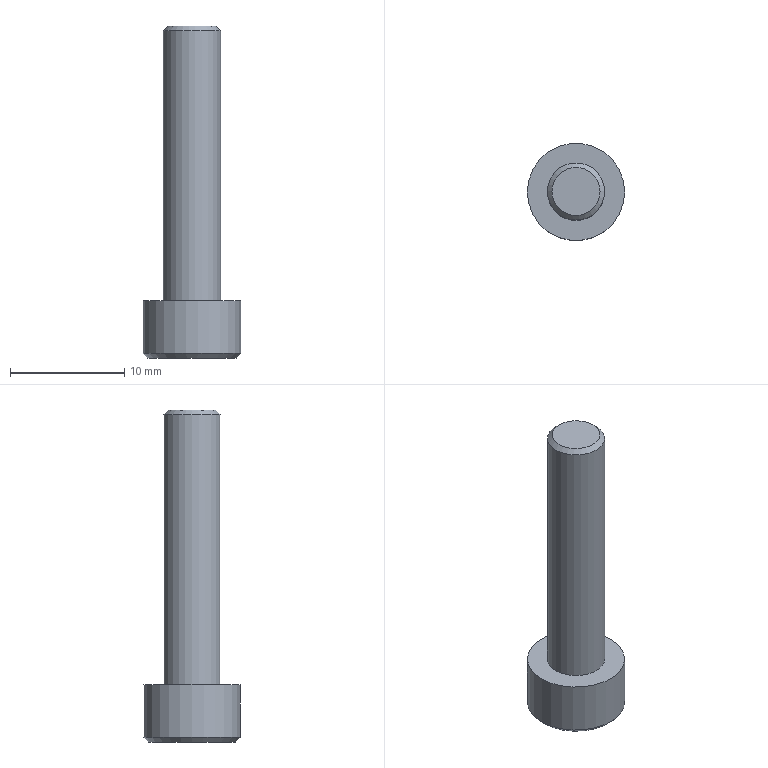Part | STEP file | M5.00-30.00 | 1 solid | 14 faces | box 8.5 x 8.5 x 29 mm | volume 713.513 mm3 | plane 10 | cylinder 2 | cone 2 | commonest cylinder face diameters 5 x1 8.5 x1